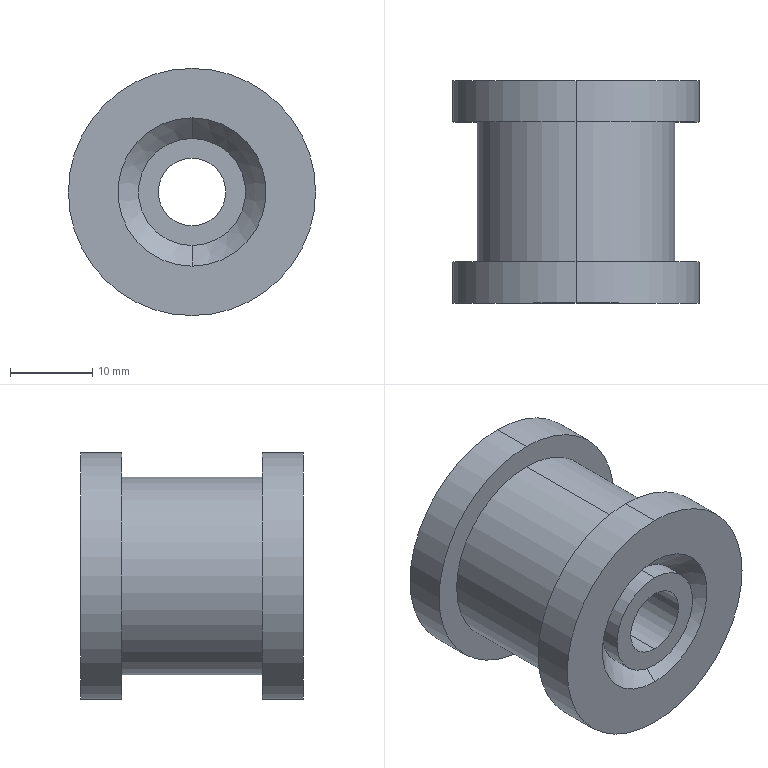Part | STEP file | B drag chain wheel | 1 solid | 22 faces | box 30 x 27 x 30 mm | volume 13045 mm3 | cylinder 12 | plane 6 | cone 4 | commonest cylinder face diameters 13 x4 30 x4 8.2 x2 24 x2
STEP:
#1=CARTESIAN_POINT('',(0.,0.,0.));
#2=DIRECTION('',(0.,0.,1.));
#3=DIRECTION('',(1.,0.,0.));
#4=AXIS2_PLACEMENT_3D('',#1,#2,#3);
#5=CARTESIAN_POINT('',(0.,27.,-4.1));
#6=VERTEX_POINT('',#5);
#7=CARTESIAN_POINT('',(0.,0.,-4.1));
#8=VERTEX_POINT('',#7);
#9=CARTESIAN_POINT('',(0.,41.,-4.1));
#10=DIRECTION('',(0.,-1.,0.));
#11=VECTOR('',#10,1.);
#12=LINE('',#9,#11);
#13=CARTESIAN_POINT('',(0.,41.,0.));
#14=DIRECTION('',(0.,-1.,0.));
#15=DIRECTION('',(0.,0.,-1.));
#16=AXIS2_PLACEMENT_3D('',#13,#14,#15);
#17=CYLINDRICAL_SURFACE('',#16,4.1);
#18=CARTESIAN_POINT('',(6.283,0.));
#19=DIRECTION('',(0.,1.));
#20=VECTOR('',#19,1.);
#21=LINE('',#18,#20);
#22=(GEOMETRIC_REPRESENTATION_CONTEXT(2)PARAMETRIC_REPRESENTATION_CONTEXT()REPRESENTATION_CONTEXT('',''));
#23=DEFINITIONAL_REPRESENTATION('',(#21),#22);
#24=PCURVE('',#17,#23);
#25=CARTESIAN_POINT('',(0.,41.,0.));
#26=DIRECTION('',(0.,-1.,0.));
#27=DIRECTION('',(0.,0.,-1.));
#28=AXIS2_PLACEMENT_3D('',#25,#26,#27);
#29=CYLINDRICAL_SURFACE('',#28,4.1);
#30=CARTESIAN_POINT('',(0.,0.));
#31=DIRECTION('',(0.,1.));
#32=VECTOR('',#31,1.);
#33=LINE('',#30,#32);
#34=(GEOMETRIC_REPRESENTATION_CONTEXT(2)PARAMETRIC_REPRESENTATION_CONTEXT()REPRESENTATION_CONTEXT('',''));
#35=DEFINITIONAL_REPRESENTATION('',(#33),#34);
#36=PCURVE('',#29,#35);
#37=SURFACE_CURVE('',#12,(#24,#36),.PCURVE_S1.);
#38=EDGE_CURVE('',#6,#8,#37,.T.);
#39=ORIENTED_EDGE('',*,*,#38,.T.);
#40=CARTESIAN_POINT('',(0.,0.,4.1));
#41=VERTEX_POINT('',#40);
#42=CARTESIAN_POINT('',(0.,0.,0.));
#43=DIRECTION('',(0.,-1.,0.));
#44=DIRECTION('',(0.,0.,-1.));
#45=AXIS2_PLACEMENT_3D('',#42,#43,#44);
#46=CIRCLE('',#45,4.1);
#47=CARTESIAN_POINT('',(0.,41.));
#48=DIRECTION('',(1.,0.));
#49=VECTOR('',#48,1.);
#50=LINE('',#47,#49);
#51=(GEOMETRIC_REPRESENTATION_CONTEXT(2)PARAMETRIC_REPRESENTATION_CONTEXT()REPRESENTATION_CONTEXT('',''));
#52=DEFINITIONAL_REPRESENTATION('',(#50),#51);
#53=PCURVE('',#17,#52);
#54=CARTESIAN_POINT('',(0.,0.,0.));
#55=DIRECTION('',(0.,-1.,0.));
#56=DIRECTION('',(0.,0.,-1.));
#57=AXIS2_PLACEMENT_3D('',#54,#55,#56);
#58=PLANE('',#57);
#59=CARTESIAN_POINT('',(0.,0.));
#60=DIRECTION('',(1.,0.));
#61=AXIS2_PLACEMENT_2D('',#59,#60);
#62=CIRCLE('',#61,4.1);
#63=(GEOMETRIC_REPRESENTATION_CONTEXT(2)PARAMETRIC_REPRESENTATION_CONTEXT()REPRESENTATION_CONTEXT('',''));
#64=DEFINITIONAL_REPRESENTATION('',(#62),#63);
#65=PCURVE('',#58,#64);
#66=SURFACE_CURVE('',#46,(#53,#65),.PCURVE_S1.);
#67=EDGE_CURVE('',#41,#8,#66,.T.);
#68=ORIENTED_EDGE('',*,*,#67,.F.);
#69=CARTESIAN_POINT('',(0.,27.,4.1));
#70=VERTEX_POINT('',#69);
#71=CARTESIAN_POINT('',(0.,41.,4.1));
#72=DIRECTION('',(0.,-1.,0.));
#73=VECTOR('',#72,1.);
#74=LINE('',#71,#73);
#75=CARTESIAN_POINT('',(3.142,0.));
#76=DIRECTION('',(0.,1.));
#77=VECTOR('',#76,1.);
#78=LINE('',#75,#77);
#79=(GEOMETRIC_REPRESENTATION_CONTEXT(2)PARAMETRIC_REPRESENTATION_CONTEXT()REPRESENTATION_CONTEXT('',''));
#80=DEFINITIONAL_REPRESENTATION('',(#78),#79);
#81=PCURVE('',#17,#80);
#82=CARTESIAN_POINT('',(3.142,0.));
#83=DIRECTION('',(0.,1.));
#84=VECTOR('',#83,1.);
#85=LINE('',#82,#84);
#86=(GEOMETRIC_REPRESENTATION_CONTEXT(2)PARAMETRIC_REPRESENTATION_CONTEXT()REPRESENTATION_CONTEXT('',''));
#87=DEFINITIONAL_REPRESENTATION('',(#85),#86);
#88=PCURVE('',#29,#87);
#89=SURFACE_CURVE('',#74,(#81,#88),.PCURVE_S1.);
#90=EDGE_CURVE('',#70,#41,#89,.T.);
#91=ORIENTED_EDGE('',*,*,#90,.F.);
#92=CARTESIAN_POINT('',(0.,27.,0.));
#93=DIRECTION('',(0.,1.,0.));
#94=DIRECTION('',(0.,0.,1.));
#95=AXIS2_PLACEMENT_3D('',#92,#93,#94);
#96=CIRCLE('',#95,4.1);
#97=CARTESIAN_POINT('',(9.425,14.));
#98=DIRECTION('',(-1.,0.));
#99=VECTOR('',#98,1.);
#100=LINE('',#97,#99);
#101=(GEOMETRIC_REPRESENTATION_CONTEXT(2)PARAMETRIC_REPRESENTATION_CONTEXT()REPRESENTATION_CONTEXT('',''));
#102=DEFINITIONAL_REPRESENTATION('',(#100),#101);
#103=PCURVE('',#17,#102);
#104=CARTESIAN_POINT('',(0.,27.,0.));
#105=DIRECTION('',(0.,1.,0.));
#106=DIRECTION('',(0.,0.,1.));
#107=AXIS2_PLACEMENT_3D('',#104,#105,#106);
#108=PLANE('',#107);
#109=CARTESIAN_POINT('',(0.,0.));
#110=DIRECTION('',(1.,0.));
#111=AXIS2_PLACEMENT_2D('',#109,#110);
#112=CIRCLE('',#111,4.1);
#113=(GEOMETRIC_REPRESENTATION_CONTEXT(2)PARAMETRIC_REPRESENTATION_CONTEXT()REPRESENTATION_CONTEXT('',''));
#114=DEFINITIONAL_REPRESENTATION('',(#112),#113);
#115=PCURVE('',#108,#114);
#116=SURFACE_CURVE('',#96,(#103,#115),.PCURVE_S1.);
#117=EDGE_CURVE('',#6,#70,#116,.T.);
#118=ORIENTED_EDGE('',*,*,#117,.F.);
#119=EDGE_LOOP('',(#39,#68,#91,#118));
#120=FACE_BOUND('',#119,.F.);
#121=ADVANCED_FACE('',(#120),#17,.F.);
#122=CARTESIAN_POINT('',(0.,27.,-6.5));
#123=VERTEX_POINT('',#122);
#124=CARTESIAN_POINT('',(0.,27.,6.5));
#125=VERTEX_POINT('',#124);
#126=CARTESIAN_POINT('',(0.,27.,0.));
#127=DIRECTION('',(0.,-1.,0.));
#128=DIRECTION('',(0.,0.,1.));
#129=AXIS2_PLACEMENT_3D('',#126,#127,#128);
#130=CIRCLE('',#129,6.5);
#131=CARTESIAN_POINT('',(0.,45.385,0.));
#132=DIRECTION('',(0.,-1.,0.));
#133=DIRECTION('',(0.,0.,-1.));
#134=AXIS2_PLACEMENT_3D('',#131,#132,#133);
#135=CYLINDRICAL_SURFACE('',#134,6.5);
#136=CARTESIAN_POINT('',(-3.142,18.385));
#137=DIRECTION('',(1.,0.));
#138=VECTOR('',#137,1.);
#139=LINE('',#136,#138);
#140=(GEOMETRIC_REPRESENTATION_CONTEXT(2)PARAMETRIC_REPRESENTATION_CONTEXT()REPRESENTATION_CONTEXT('',''));
#141=DEFINITIONAL_REPRESENTATION('',(#139),#140);
#142=PCURVE('',#135,#141);
#143=CARTESIAN_POINT('',(6.5,0.));
#144=CARTESIAN_POINT('',(6.5,-11.258));
#145=CARTESIAN_POINT('',(-3.25,-5.629));
#146=CARTESIAN_POINT('',(-13.,0.));
#147=CARTESIAN_POINT('',(-3.25,5.629));
#148=CARTESIAN_POINT('',(6.5,11.258));
#149=CARTESIAN_POINT('',(6.5,0.));
#150=(BOUNDED_CURVE()B_SPLINE_CURVE(2,(#143,#144,#145,#146,#147,#148,#149),.UNSPECIFIED.,.T.,.F.)B_SPLINE_CURVE_WITH_KNOTS((1,2,2,2,2,1),(-2.094,0.,2.094,4.189,6.283,8.378),.UNSPECIFIED.)CURVE()GEOMETRIC_REPRESENTATION_ITEM()RATIONAL_B_SPLINE_CURVE((1.,0.5,1.,0.5,1.,0.5,1.))REPRESENTATION_ITEM(''));
#151=(GEOMETRIC_REPRESENTATION_CONTEXT(2)PARAMETRIC_REPRESENTATION_CONTEXT()REPRESENTATION_CONTEXT('',''));
#152=DEFINITIONAL_REPRESENTATION('',(#150),#151);
#153=PCURVE('',#108,#152);
#154=SURFACE_CURVE('',#130,(#142,#153),.PCURVE_S1.);
#155=EDGE_CURVE('',#123,#125,#154,.T.);
#156=ORIENTED_EDGE('',*,*,#155,.T.);
#157=CARTESIAN_POINT('',(0.,24.5,6.5));
#158=VERTEX_POINT('',#157);
#159=CARTESIAN_POINT('',(0.,45.385,6.5));
#160=DIRECTION('',(0.,-1.,0.));
#161=VECTOR('',#160,1.);
#162=LINE('',#159,#161);
#163=CARTESIAN_POINT('',(3.142,0.));
#164=DIRECTION('',(0.,1.));
#165=VECTOR('',#164,1.);
#166=LINE('',#163,#165);
#167=(GEOMETRIC_REPRESENTATION_CONTEXT(2)PARAMETRIC_REPRESENTATION_CONTEXT()REPRESENTATION_CONTEXT('',''));
#168=DEFINITIONAL_REPRESENTATION('',(#166),#167);
#169=PCURVE('',#135,#168);
#170=CARTESIAN_POINT('',(0.,45.385,0.));
#171=DIRECTION('',(0.,-1.,0.));
#172=DIRECTION('',(0.,0.,-1.));
#173=AXIS2_PLACEMENT_3D('',#170,#171,#172);
#174=CYLINDRICAL_SURFACE('',#173,6.5);
#175=CARTESIAN_POINT('',(3.142,0.));
#176=DIRECTION('',(0.,1.));
#177=VECTOR('',#176,1.);
#178=LINE('',#175,#177);
#179=(GEOMETRIC_REPRESENTATION_CONTEXT(2)PARAMETRIC_REPRESENTATION_CONTEXT()REPRESENTATION_CONTEXT('',''));
#180=DEFINITIONAL_REPRESENTATION('',(#178),#179);
#181=PCURVE('',#174,#180);
#182=SURFACE_CURVE('',#162,(#169,#181),.PCURVE_S1.);
#183=EDGE_CURVE('',#125,#158,#182,.T.);
#184=ORIENTED_EDGE('',*,*,#183,.T.);
#185=CARTESIAN_POINT('',(0.,24.5,-6.5));
#186=VERTEX_POINT('',#185);
#187=CARTESIAN_POINT('',(0.,24.5,0.));
#188=DIRECTION('',(0.,1.,0.));
#189=DIRECTION('',(0.,0.,1.));
#190=AXIS2_PLACEMENT_3D('',#187,#188,#189);
#191=CIRCLE('',#190,6.5);
#192=CARTESIAN_POINT('',(3.142,20.885));
#193=DIRECTION('',(-1.,0.));
#194=VECTOR('',#193,1.);
#195=LINE('',#192,#194);
#196=(GEOMETRIC_REPRESENTATION_CONTEXT(2)PARAMETRIC_REPRESENTATION_CONTEXT()REPRESENTATION_CONTEXT('',''));
#197=DEFINITIONAL_REPRESENTATION('',(#195),#196);
#198=PCURVE('',#135,#197);
#199=CARTESIAN_POINT('',(0.,22.,0.));
#200=DIRECTION('',(0.,1.,0.));
#201=DIRECTION('',(0.,0.,1.));
#202=AXIS2_PLACEMENT_3D('',#199,#200,#201);
#203=CONICAL_SURFACE('',#202,4.,0.7854);
#204=CARTESIAN_POINT('',(0.,2.5));
#205=DIRECTION('',(1.,0.));
#206=VECTOR('',#205,1.);
#207=LINE('',#204,#206);
#208=(GEOMETRIC_REPRESENTATION_CONTEXT(2)PARAMETRIC_REPRESENTATION_CONTEXT()REPRESENTATION_CONTEXT('',''));
#209=DEFINITIONAL_REPRESENTATION('',(#207),#208);
#210=PCURVE('',#203,#209);
#211=SURFACE_CURVE('',#191,(#198,#210),.PCURVE_S1.);
#212=EDGE_CURVE('',#158,#186,#211,.T.);
#213=ORIENTED_EDGE('',*,*,#212,.T.);
#214=CARTESIAN_POINT('',(0.,45.385,-6.5));
#215=DIRECTION('',(0.,-1.,0.));
#216=VECTOR('',#215,1.);
#217=LINE('',#214,#216);
#218=CARTESIAN_POINT('',(0.,0.));
#219=DIRECTION('',(0.,1.));
#220=VECTOR('',#219,1.);
#221=LINE('',#218,#220);
#222=(GEOMETRIC_REPRESENTATION_CONTEXT(2)PARAMETRIC_REPRESENTATION_CONTEXT()REPRESENTATION_CONTEXT('',''));
#223=DEFINITIONAL_REPRESENTATION('',(#221),#222);
#224=PCURVE('',#135,#223);
#225=CARTESIAN_POINT('',(6.283,0.));
#226=DIRECTION('',(0.,1.));
#227=VECTOR('',#226,1.);
#228=LINE('',#225,#227);
#229=(GEOMETRIC_REPRESENTATION_CONTEXT(2)PARAMETRIC_REPRESENTATION_CONTEXT()REPRESENTATION_CONTEXT('',''));
#230=DEFINITIONAL_REPRESENTATION('',(#228),#229);
#231=PCURVE('',#174,#230);
#232=SURFACE_CURVE('',#217,(#224,#231),.PCURVE_S1.);
#233=EDGE_CURVE('',#123,#186,#232,.T.);
#234=ORIENTED_EDGE('',*,*,#233,.F.);
#235=EDGE_LOOP('',(#156,#184,#213,#234));
#236=FACE_BOUND('',#235,.T.);
#237=ADVANCED_FACE('',(#236),#135,.T.);
#238=CARTESIAN_POINT('',(0.,2.5,-6.5));
#239=VERTEX_POINT('',#238);
#240=CARTESIAN_POINT('',(0.,2.5,6.5));
#241=VERTEX_POINT('',#240);
#242=CARTESIAN_POINT('',(0.,2.5,0.));
#243=DIRECTION('',(0.,-1.,0.));
#244=DIRECTION('',(0.,0.,-1.));
#245=AXIS2_PLACEMENT_3D('',#242,#243,#244);
#246=CIRCLE('',#245,6.5);
#247=CARTESIAN_POINT('',(0.,45.385,0.));
#248=DIRECTION('',(0.,-1.,0.));
#249=DIRECTION('',(0.,0.,-1.));
#250=AXIS2_PLACEMENT_3D('',#247,#248,#249);
#251=CYLINDRICAL_SURFACE('',#250,6.5);
#252=CARTESIAN_POINT('',(0.,42.885));
#253=DIRECTION('',(1.,0.));
#254=VECTOR('',#253,1.);
#255=LINE('',#252,#254);
#256=(GEOMETRIC_REPRESENTATION_CONTEXT(2)PARAMETRIC_REPRESENTATION_CONTEXT()REPRESENTATION_CONTEXT('',''));
#257=DEFINITIONAL_REPRESENTATION('',(#255),#256);
#258=PCURVE('',#251,#257);
#259=CARTESIAN_POINT('',(0.,5.,0.));
#260=DIRECTION('',(0.,-1.,0.));
#261=DIRECTION('',(0.,0.,-1.));
#262=AXIS2_PLACEMENT_3D('',#259,#260,#261);
#263=CONICAL_SURFACE('',#262,4.,0.7854);
#264=CARTESIAN_POINT('',(0.,2.5));
#265=DIRECTION('',(1.,0.));
#266=VECTOR('',#265,1.);
#267=LINE('',#264,#266);
#268=(GEOMETRIC_REPRESENTATION_CONTEXT(2)PARAMETRIC_REPRESENTATION_CONTEXT()REPRESENTATION_CONTEXT('',''));
#269=DEFINITIONAL_REPRESENTATION('',(#267),#268);
#270=PCURVE('',#263,#269);
#271=SURFACE_CURVE('',#246,(#258,#270),.PCURVE_S1.);
#272=EDGE_CURVE('',#239,#241,#271,.T.);
#273=ORIENTED_EDGE('',*,*,#272,.T.);
#274=CARTESIAN_POINT('',(0.,0.,6.5));
#275=VERTEX_POINT('',#274);
#276=CARTESIAN_POINT('',(0.,45.385,6.5));
#277=DIRECTION('',(0.,-1.,0.));
#278=VECTOR('',#277,1.);
#279=LINE('',#276,#278);
#280=CARTESIAN_POINT('',(3.142,0.));
#281=DIRECTION('',(0.,1.));
#282=VECTOR('',#281,1.);
#283=LINE('',#280,#282);
#284=(GEOMETRIC_REPRESENTATION_CONTEXT(2)PARAMETRIC_REPRESENTATION_CONTEXT()REPRESENTATION_CONTEXT('',''));
#285=DEFINITIONAL_REPRESENTATION('',(#283),#284);
#286=PCURVE('',#251,#285);
#287=CARTESIAN_POINT('',(0.,45.385,0.));
#288=DIRECTION('',(0.,-1.,0.));
#289=DIRECTION('',(0.,0.,-1.));
#290=AXIS2_PLACEMENT_3D('',#287,#288,#289);
#291=CYLINDRICAL_SURFACE('',#290,6.5);
#292=CARTESIAN_POINT('',(3.142,0.));
#293=DIRECTION('',(0.,1.));
#294=VECTOR('',#293,1.);
#295=LINE('',#292,#294);
#296=(GEOMETRIC_REPRESENTATION_CONTEXT(2)PARAMETRIC_REPRESENTATION_CONTEXT()REPRESENTATION_CONTEXT('',''));
#297=DEFINITIONAL_REPRESENTATION('',(#295),#296);
#298=PCURVE('',#291,#297);
#299=SURFACE_CURVE('',#279,(#286,#298),.PCURVE_S1.);
#300=EDGE_CURVE('',#241,#275,#299,.T.);
#301=ORIENTED_EDGE('',*,*,#300,.T.);
#302=CARTESIAN_POINT('',(0.,0.,-6.5));
#303=VERTEX_POINT('',#302);
#304=CARTESIAN_POINT('',(0.,0.,0.));
#305=DIRECTION('',(0.,-1.,0.));
#306=DIRECTION('',(0.,0.,-1.));
#307=AXIS2_PLACEMENT_3D('',#304,#305,#306);
#308=CIRCLE('',#307,6.5);
#309=CARTESIAN_POINT('',(0.,45.385));
#310=DIRECTION('',(1.,0.));
#311=VECTOR('',#310,1.);
#312=LINE('',#309,#311);
#313=(GEOMETRIC_REPRESENTATION_CONTEXT(2)PARAMETRIC_REPRESENTATION_CONTEXT()REPRESENTATION_CONTEXT('',''));
#314=DEFINITIONAL_REPRESENTATION('',(#312),#313);
#315=PCURVE('',#251,#314);
#316=CARTESIAN_POINT('',(0.,0.));
#317=DIRECTION('',(1.,0.));
#318=AXIS2_PLACEMENT_2D('',#316,#317);
#319=CIRCLE('',#318,6.5);
#320=(GEOMETRIC_REPRESENTATION_CONTEXT(2)PARAMETRIC_REPRESENTATION_CONTEXT()REPRESENTATION_CONTEXT('',''));
#321=DEFINITIONAL_REPRESENTATION('',(#319),#320);
#322=PCURVE('',#58,#321);
#323=SURFACE_CURVE('',#308,(#315,#322),.PCURVE_S1.);
#324=EDGE_CURVE('',#303,#275,#323,.T.);
#325=ORIENTED_EDGE('',*,*,#324,.F.);
#326=CARTESIAN_POINT('',(0.,45.385,-6.5));
#327=DIRECTION('',(0.,-1.,0.));
#328=VECTOR('',#327,1.);
#329=LINE('',#326,#328);
#330=CARTESIAN_POINT('',(0.,0.));
#331=DIRECTION('',(0.,1.));
#332=VECTOR('',#331,1.);
#333=LINE('',#330,#332);
#334=(GEOMETRIC_REPRESENTATION_CONTEXT(2)PARAMETRIC_REPRESENTATION_CONTEXT()REPRESENTATION_CONTEXT('',''));
#335=DEFINITIONAL_REPRESENTATION('',(#333),#334);
#336=PCURVE('',#251,#335);
#337=CARTESIAN_POINT('',(6.283,0.));
#338=DIRECTION('',(0.,1.));
#339=VECTOR('',#338,1.);
#340=LINE('',#337,#339);
#341=(GEOMETRIC_REPRESENTATION_CONTEXT(2)PARAMETRIC_REPRESENTATION_CONTEXT()REPRESENTATION_CONTEXT('',''));
#342=DEFINITIONAL_REPRESENTATION('',(#340),#341);
#343=PCURVE('',#291,#342);
#344=SURFACE_CURVE('',#329,(#336,#343),.PCURVE_S1.);
#345=EDGE_CURVE('',#239,#303,#344,.T.);
#346=ORIENTED_EDGE('',*,*,#345,.F.);
#347=EDGE_LOOP('',(#273,#301,#325,#346));
#348=FACE_BOUND('',#347,.T.);
#349=ADVANCED_FACE('',(#348),#251,.T.);
#350=CARTESIAN_POINT('',(0.,27.,9.));
#351=VERTEX_POINT('',#350);
#352=CARTESIAN_POINT('',(0.,22.,4.));
#353=DIRECTION('',(0.,0.7071,0.7071));
#354=VECTOR('',#353,1.);
#355=LINE('',#352,#354);
#356=CARTESIAN_POINT('',(0.,22.,0.));
#357=DIRECTION('',(0.,1.,0.));
#358=DIRECTION('',(0.,0.,1.));
#359=AXIS2_PLACEMENT_3D('',#356,#357,#358);
#360=CONICAL_SURFACE('',#359,4.,0.7854);
#361=CARTESIAN_POINT('',(6.283,0.));
#362=DIRECTION('',(0.,1.));
#363=VECTOR('',#362,1.);
#364=LINE('',#361,#363);
#365=(GEOMETRIC_REPRESENTATION_CONTEXT(2)PARAMETRIC_REPRESENTATION_CONTEXT()REPRESENTATION_CONTEXT('',''));
#366=DEFINITIONAL_REPRESENTATION('',(#364),#365);
#367=PCURVE('',#360,#366);
#368=CARTESIAN_POINT('',(0.,0.));
#369=DIRECTION('',(0.,1.));
#370=VECTOR('',#369,1.);
#371=LINE('',#368,#370);
#372=(GEOMETRIC_REPRESENTATION_CONTEXT(2)PARAMETRIC_REPRESENTATION_CONTEXT()REPRESENTATION_CONTEXT('',''));
#373=DEFINITIONAL_REPRESENTATION('',(#371),#372);
#374=PCURVE('',#203,#373);
#375=SURFACE_CURVE('',#355,(#367,#374),.PCURVE_S1.);
#376=EDGE_CURVE('',#158,#351,#375,.T.);
#377=ORIENTED_EDGE('',*,*,#376,.T.);
#378=CARTESIAN_POINT('',(0.,27.,-9.));
#379=VERTEX_POINT('',#378);
#380=CARTESIAN_POINT('',(0.,27.,0.));
#381=DIRECTION('',(0.,-1.,0.));
#382=DIRECTION('',(0.,0.,1.));
#383=AXIS2_PLACEMENT_3D('',#380,#381,#382);
#384=CIRCLE('',#383,9.);
#385=CARTESIAN_POINT('',(6.283,5.));
#386=DIRECTION('',(-1.,0.));
#387=VECTOR('',#386,1.);
#388=LINE('',#385,#387);
#389=(GEOMETRIC_REPRESENTATION_CONTEXT(2)PARAMETRIC_REPRESENTATION_CONTEXT()REPRESENTATION_CONTEXT('',''));
#390=DEFINITIONAL_REPRESENTATION('',(#388),#389);
#391=PCURVE('',#360,#390);
#392=CARTESIAN_POINT('',(0.,27.,0.));
#393=DIRECTION('',(0.,1.,0.));
#394=DIRECTION('',(0.,0.,1.));
#395=AXIS2_PLACEMENT_3D('',#392,#393,#394);
#396=PLANE('',#395);
#397=CARTESIAN_POINT('',(9.,0.));
#398=CARTESIAN_POINT('',(9.,-15.588));
#399=CARTESIAN_POINT('',(-4.5,-7.794));
#400=CARTESIAN_POINT('',(-18.,0.));
#401=CARTESIAN_POINT('',(-4.5,7.794));
#402=CARTESIAN_POINT('',(9.,15.588));
#403=CARTESIAN_POINT('',(9.,0.));
#404=(BOUNDED_CURVE()B_SPLINE_CURVE(2,(#397,#398,#399,#400,#401,#402,#403),.UNSPECIFIED.,.T.,.F.)B_SPLINE_CURVE_WITH_KNOTS((1,2,2,2,2,1),(-2.094,0.,2.094,4.189,6.283,8.378),.UNSPECIFIED.)CURVE()GEOMETRIC_REPRESENTATION_ITEM()RATIONAL_B_SPLINE_CURVE((1.,0.5,1.,0.5,1.,0.5,1.))REPRESENTATION_ITEM(''));
#405=(GEOMETRIC_REPRESENTATION_CONTEXT(2)PARAMETRIC_REPRESENTATION_CONTEXT()REPRESENTATION_CONTEXT('',''));
#406=DEFINITIONAL_REPRESENTATION('',(#404),#405);
#407=PCURVE('',#396,#406);
#408=SURFACE_CURVE('',#384,(#391,#407),.PCURVE_S1.);
#409=EDGE_CURVE('',#351,#379,#408,.T.);
#410=ORIENTED_EDGE('',*,*,#409,.T.);
#411=CARTESIAN_POINT('',(0.,22.,-4.));
#412=DIRECTION('',(0.,0.7071,-0.7071));
#413=VECTOR('',#412,1.);
#414=LINE('',#411,#413);
#415=CARTESIAN_POINT('',(3.142,0.));
#416=DIRECTION('',(0.,1.));
#417=VECTOR('',#416,1.);
#418=LINE('',#415,#417);
#419=(GEOMETRIC_REPRESENTATION_CONTEXT(2)PARAMETRIC_REPRESENTATION_CONTEXT()REPRESENTATION_CONTEXT('',''));
#420=DEFINITIONAL_REPRESENTATION('',(#418),#419);
#421=PCURVE('',#360,#420);
#422=CARTESIAN_POINT('',(3.142,0.));
#423=DIRECTION('',(0.,1.));
#424=VECTOR('',#423,1.);
#425=LINE('',#422,#424);
#426=(GEOMETRIC_REPRESENTATION_CONTEXT(2)PARAMETRIC_REPRESENTATION_CONTEXT()REPRESENTATION_CONTEXT('',''));
#427=DEFINITIONAL_REPRESENTATION('',(#425),#426);
#428=PCURVE('',#203,#427);
#429=SURFACE_CURVE('',#414,(#421,#428),.PCURVE_S1.);
#430=EDGE_CURVE('',#186,#379,#429,.T.);
#431=ORIENTED_EDGE('',*,*,#430,.F.);
#432=CARTESIAN_POINT('',(0.,24.5,0.));
#433=DIRECTION('',(0.,1.,0.));
#434=DIRECTION('',(0.,0.,1.));
#435=AXIS2_PLACEMENT_3D('',#432,#433,#434);
#436=CIRCLE('',#435,6.5);
#437=CARTESIAN_POINT('',(0.,2.5));
#438=DIRECTION('',(1.,0.));
#439=VECTOR('',#438,1.);
#440=LINE('',#437,#439);
#441=(GEOMETRIC_REPRESENTATION_CONTEXT(2)PARAMETRIC_REPRESENTATION_CONTEXT()REPRESENTATION_CONTEXT('',''));
#442=DEFINITIONAL_REPRESENTATION('',(#440),#441);
#443=PCURVE('',#360,#442);
#444=CARTESIAN_POINT('',(9.425,20.885));
#445=DIRECTION('',(-1.,0.));
#446=VECTOR('',#445,1.);
#447=LINE('',#444,#446);
#448=(GEOMETRIC_REPRESENTATION_CONTEXT(2)PARAMETRIC_REPRESENTATION_CONTEXT()REPRESENTATION_CONTEXT('',''));
#449=DEFINITIONAL_REPRESENTATION('',(#447),#448);
#450=PCURVE('',#174,#449);
#451=SURFACE_CURVE('',#436,(#443,#450),.PCURVE_S1.);
#452=EDGE_CURVE('',#186,#158,#451,.T.);
#453=ORIENTED_EDGE('',*,*,#452,.T.);
#454=EDGE_LOOP('',(#377,#410,#431,#453));
#455=FACE_BOUND('',#454,.F.);
#456=ADVANCED_FACE('',(#455),#360,.F.);
#457=CARTESIAN_POINT('',(0.,0.,-9.));
#458=VERTEX_POINT('',#457);
#459=CARTESIAN_POINT('',(0.,5.,-4.));
#460=DIRECTION('',(0.,-0.7071,-0.7071));
#461=VECTOR('',#460,1.);
#462=LINE('',#459,#461);
#463=CARTESIAN_POINT('',(0.,5.,0.));
#464=DIRECTION('',(0.,-1.,0.));
#465=DIRECTION('',(0.,0.,-1.));
#466=AXIS2_PLACEMENT_3D('',#463,#464,#465);
#467=CONICAL_SURFACE('',#466,4.,0.7854);
#468=CARTESIAN_POINT('',(6.283,0.));
#469=DIRECTION('',(0.,1.));
#470=VECTOR('',#469,1.);
#471=LINE('',#468,#470);
#472=(GEOMETRIC_REPRESENTATION_CONTEXT(2)PARAMETRIC_REPRESENTATION_CONTEXT()REPRESENTATION_CONTEXT('',''));
#473=DEFINITIONAL_REPRESENTATION('',(#471),#472);
#474=PCURVE('',#467,#473);
#475=CARTESIAN_POINT('',(0.,0.));
#476=DIRECTION('',(0.,1.));
#477=VECTOR('',#476,1.);
#478=LINE('',#475,#477);
#479=(GEOMETRIC_REPRESENTATION_CONTEXT(2)PARAMETRIC_REPRESENTATION_CONTEXT()REPRESENTATION_CONTEXT('',''));
#480=DEFINITIONAL_REPRESENTATION('',(#478),#479);
#481=PCURVE('',#263,#480);
#482=SURFACE_CURVE('',#462,(#474,#481),.PCURVE_S1.);
#483=EDGE_CURVE('',#239,#458,#482,.T.);
#484=ORIENTED_EDGE('',*,*,#483,.T.);
#485=CARTESIAN_POINT('',(0.,0.,9.));
#486=VERTEX_POINT('',#485);
#487=CARTESIAN_POINT('',(0.,0.,0.));
#488=DIRECTION('',(0.,1.,0.));
#489=DIRECTION('',(0.,0.,1.));
#490=AXIS2_PLACEMENT_3D('',#487,#488,#489);
#491=CIRCLE('',#490,9.);
#492=CARTESIAN_POINT('',(9.425,5.));
#493=DIRECTION('',(-1.,0.));
#494=VECTOR('',#493,1.);
#495=LINE('',#492,#494);
#496=(GEOMETRIC_REPRESENTATION_CONTEXT(2)PARAMETRIC_REPRESENTATION_CONTEXT()REPRESENTATION_CONTEXT('',''));
#497=DEFINITIONAL_REPRESENTATION('',(#495),#496);
#498=PCURVE('',#467,#497);
#499=CARTESIAN_POINT('',(0.,0.,0.));
#500=DIRECTION('',(0.,1.,0.));
#501=DIRECTION('',(0.,0.,1.));
#502=AXIS2_PLACEMENT_3D('',#499,#500,#501);
#503=PLANE('',#502);
#504=CARTESIAN_POINT('',(0.,0.));
#505=DIRECTION('',(1.,0.));
#506=AXIS2_PLACEMENT_2D('',#504,#505);
#507=CIRCLE('',#506,9.);
#508=(GEOMETRIC_REPRESENTATION_CONTEXT(2)PARAMETRIC_REPRESENTATION_CONTEXT()REPRESENTATION_CONTEXT('',''));
#509=DEFINITIONAL_REPRESENTATION('',(#507),#508);
#510=PCURVE('',#503,#509);
#511=SURFACE_CURVE('',#491,(#498,#510),.PCURVE_S1.);
#512=EDGE_CURVE('',#458,#486,#511,.T.);
#513=ORIENTED_EDGE('',*,*,#512,.T.);
#514=CARTESIAN_POINT('',(0.,5.,4.));
#515=DIRECTION('',(0.,-0.7071,0.7071));
#516=VECTOR('',#515,1.);
#517=LINE('',#514,#516);
#518=CARTESIAN_POINT('',(3.142,0.));
#519=DIRECTION('',(0.,1.));
#520=VECTOR('',#519,1.);
#521=LINE('',#518,#520);
#522=(GEOMETRIC_REPRESENTATION_CONTEXT(2)PARAMETRIC_REPRESENTATION_CONTEXT()REPRESENTATION_CONTEXT('',''));
#523=DEFINITIONAL_REPRESENTATION('',(#521),#522);
#524=PCURVE('',#467,#523);
#525=CARTESIAN_POINT('',(3.142,0.));
#526=DIRECTION('',(0.,1.));
#527=VECTOR('',#526,1.);
#528=LINE('',#525,#527);
#529=(GEOMETRIC_REPRESENTATION_CONTEXT(2)PARAMETRIC_REPRESENTATION_CONTEXT()REPRESENTATION_CONTEXT('',''));
#530=DEFINITIONAL_REPRESENTATION('',(#528),#529);
#531=PCURVE('',#263,#530);
#532=SURFACE_CURVE('',#517,(#524,#531),.PCURVE_S1.);
#533=EDGE_CURVE('',#241,#486,#532,.T.);
#534=ORIENTED_EDGE('',*,*,#533,.F.);
#535=CARTESIAN_POINT('',(0.,2.5,0.));
#536=DIRECTION('',(0.,-1.,0.));
#537=DIRECTION('',(0.,0.,-1.));
#538=AXIS2_PLACEMENT_3D('',#535,#536,#537);
#539=CIRCLE('',#538,6.5);
#540=CARTESIAN_POINT('',(0.,2.5));
#541=DIRECTION('',(1.,0.));
#542=VECTOR('',#541,1.);
#543=LINE('',#540,#542);
#544=(GEOMETRIC_REPRESENTATION_CONTEXT(2)PARAMETRIC_REPRESENTATION_CONTEXT()REPRESENTATION_CONTEXT('',''));
#545=DEFINITIONAL_REPRESENTATION('',(#543),#544);
#546=PCURVE('',#467,#545);
#547=CARTESIAN_POINT('',(0.,42.885));
#548=DIRECTION('',(1.,0.));
#549=VECTOR('',#548,1.);
#550=LINE('',#547,#549);
#551=(GEOMETRIC_REPRESENTATION_CONTEXT(2)PARAMETRIC_REPRESENTATION_CONTEXT()REPRESENTATION_CONTEXT('',''));
#552=DEFINITIONAL_REPRESENTATION('',(#550),#551);
#553=PCURVE('',#291,#552);
#554=SURFACE_CURVE('',#539,(#546,#553),.PCURVE_S1.);
#555=EDGE_CURVE('',#241,#239,#554,.T.);
#556=ORIENTED_EDGE('',*,*,#555,.T.);
#557=EDGE_LOOP('',(#484,#513,#534,#556));
#558=FACE_BOUND('',#557,.F.);
#559=ADVANCED_FACE('',(#558),#467,.F.);
#560=CARTESIAN_POINT('',(0.,22.,15.));
#561=VERTEX_POINT('',#560);
#562=CARTESIAN_POINT('',(0.,22.,-15.));
#563=VERTEX_POINT('',#562);
#564=CARTESIAN_POINT('',(0.,22.,0.));
#565=DIRECTION('',(0.,1.,0.));
#566=DIRECTION('',(0.,0.,1.));
#567=AXIS2_PLACEMENT_3D('',#564,#565,#566);
#568=CIRCLE('',#567,15.);
#569=CARTESIAN_POINT('',(0.,22.,0.));
#570=DIRECTION('',(0.,1.,0.));
#571=DIRECTION('',(0.,0.,1.));
#572=AXIS2_PLACEMENT_3D('',#569,#570,#571);
#573=CYLINDRICAL_SURFACE('',#572,15.);
#574=CARTESIAN_POINT('',(0.,0.));
#575=DIRECTION('',(1.,0.));
#576=VECTOR('',#575,1.);
#577=LINE('',#574,#576);
#578=(GEOMETRIC_REPRESENTATION_CONTEXT(2)PARAMETRIC_REPRESENTATION_CONTEXT()REPRESENTATION_CONTEXT('',''));
#579=DEFINITIONAL_REPRESENTATION('',(#577),#578);
#580=PCURVE('',#573,#579);
#581=CARTESIAN_POINT('',(0.,22.,0.));
#582=DIRECTION('',(0.,1.,0.));
#583=DIRECTION('',(0.,0.,1.));
#584=AXIS2_PLACEMENT_3D('',#581,#582,#583);
#585=PLANE('',#584);
#586=CARTESIAN_POINT('',(0.,0.));
#587=DIRECTION('',(1.,0.));
#588=AXIS2_PLACEMENT_2D('',#586,#587);
#589=CIRCLE('',#588,15.);
#590=(GEOMETRIC_REPRESENTATION_CONTEXT(2)PARAMETRIC_REPRESENTATION_CONTEXT()REPRESENTATION_CONTEXT('',''));
#591=DEFINITIONAL_REPRESENTATION('',(#589),#590);
#592=PCURVE('',#585,#591);
#593=SURFACE_CURVE('',#568,(#580,#592),.PCURVE_S1.);
#594=EDGE_CURVE('',#561,#563,#593,.T.);
#595=ORIENTED_EDGE('',*,*,#594,.T.);
#596=CARTESIAN_POINT('',(0.,27.,-15.));
#597=VERTEX_POINT('',#596);
#598=CARTESIAN_POINT('',(0.,22.,-15.));
#599=DIRECTION('',(0.,1.,0.));
#600=VECTOR('',#599,1.);
#601=LINE('',#598,#600);
#602=CARTESIAN_POINT('',(3.142,0.));
#603=DIRECTION('',(0.,1.));
#604=VECTOR('',#603,1.);
#605=LINE('',#602,#604);
#606=(GEOMETRIC_REPRESENTATION_CONTEXT(2)PARAMETRIC_REPRESENTATION_CONTEXT()REPRESENTATION_CONTEXT('',''));
#607=DEFINITIONAL_REPRESENTATION('',(#605),#606);
#608=PCURVE('',#573,#607);
#609=CARTESIAN_POINT('',(0.,22.,0.));
#610=DIRECTION('',(0.,1.,0.));
#611=DIRECTION('',(0.,0.,1.));
#612=AXIS2_PLACEMENT_3D('',#609,#610,#611);
#613=CYLINDRICAL_SURFACE('',#612,15.);
#614=CARTESIAN_POINT('',(3.142,0.));
#615=DIRECTION('',(0.,1.));
#616=VECTOR('',#615,1.);
#617=LINE('',#614,#616);
#618=(GEOMETRIC_REPRESENTATION_CONTEXT(2)PARAMETRIC_REPRESENTATION_CONTEXT()REPRESENTATION_CONTEXT('',''));
#619=DEFINITIONAL_REPRESENTATION('',(#617),#618);
#620=PCURVE('',#613,#619);
#621=SURFACE_CURVE('',#601,(#608,#620),.PCURVE_S1.);
#622=EDGE_CURVE('',#563,#597,#621,.T.);
#623=ORIENTED_EDGE('',*,*,#622,.T.);
#624=CARTESIAN_POINT('',(0.,27.,15.));
#625=VERTEX_POINT('',#624);
#626=CARTESIAN_POINT('',(0.,27.,0.));
#627=DIRECTION('',(0.,1.,0.));
#628=DIRECTION('',(0.,0.,1.));
#629=AXIS2_PLACEMENT_3D('',#626,#627,#628);
#630=CIRCLE('',#629,15.);
#631=CARTESIAN_POINT('',(0.,5.));
#632=DIRECTION('',(1.,0.));
#633=VECTOR('',#632,1.);
#634=LINE('',#631,#633);
#635=(GEOMETRIC_REPRESENTATION_CONTEXT(2)PARAMETRIC_REPRESENTATION_CONTEXT()REPRESENTATION_CONTEXT('',''));
#636=DEFINITIONAL_REPRESENTATION('',(#634),#635);
#637=PCURVE('',#573,#636);
#638=CARTESIAN_POINT('',(0.,0.));
#639=DIRECTION('',(1.,0.));
#640=AXIS2_PLACEMENT_2D('',#638,#639);
#641=CIRCLE('',#640,15.);
#642=(GEOMETRIC_REPRESENTATION_CONTEXT(2)PARAMETRIC_REPRESENTATION_CONTEXT()REPRESENTATION_CONTEXT('',''));
#643=DEFINITIONAL_REPRESENTATION('',(#641),#642);
#644=PCURVE('',#396,#643);
#645=SURFACE_CURVE('',#630,(#637,#644),.PCURVE_S1.);
#646=EDGE_CURVE('',#625,#597,#645,.T.);
#647=ORIENTED_EDGE('',*,*,#646,.F.);
#648=CARTESIAN_POINT('',(0.,22.,15.));
#649=DIRECTION('',(0.,1.,0.));
#650=VECTOR('',#649,1.);
#651=LINE('',#648,#650);
#652=CARTESIAN_POINT('',(0.,0.));
#653=DIRECTION('',(0.,1.));
#654=VECTOR('',#653,1.);
#655=LINE('',#652,#654);
#656=(GEOMETRIC_REPRESENTATION_CONTEXT(2)PARAMETRIC_REPRESENTATION_CONTEXT()REPRESENTATION_CONTEXT('',''));
#657=DEFINITIONAL_REPRESENTATION('',(#655),#656);
#658=PCURVE('',#573,#657);
#659=CARTESIAN_POINT('',(6.283,0.));
#660=DIRECTION('',(0.,1.));
#661=VECTOR('',#660,1.);
#662=LINE('',#659,#661);
#663=(GEOMETRIC_REPRESENTATION_CONTEXT(2)PARAMETRIC_REPRESENTATION_CONTEXT()REPRESENTATION_CONTEXT('',''));
#664=DEFINITIONAL_REPRESENTATION('',(#662),#663);
#665=PCURVE('',#613,#664);
#666=SURFACE_CURVE('',#651,(#658,#665),.PCURVE_S1.);
#667=EDGE_CURVE('',#561,#625,#666,.T.);
#668=ORIENTED_EDGE('',*,*,#667,.F.);
#669=EDGE_LOOP('',(#595,#623,#647,#668));
#670=FACE_BOUND('',#669,.T.);
#671=ADVANCED_FACE('',(#670),#573,.T.);
#672=CARTESIAN_POINT('',(0.,5.,-15.));
#673=VERTEX_POINT('',#672);
#674=CARTESIAN_POINT('',(0.,5.,15.));
#675=VERTEX_POINT('',#674);
#676=CARTESIAN_POINT('',(0.,5.,0.));
#677=DIRECTION('',(0.,-1.,0.));
#678=DIRECTION('',(0.,0.,-1.));
#679=AXIS2_PLACEMENT_3D('',#676,#677,#678);
#680=CIRCLE('',#679,15.);
#681=CARTESIAN_POINT('',(0.,5.,0.));
#682=DIRECTION('',(0.,-1.,0.));
#683=DIRECTION('',(0.,0.,-1.));
#684=AXIS2_PLACEMENT_3D('',#681,#682,#683);
#685=CYLINDRICAL_SURFACE('',#684,15.);
#686=CARTESIAN_POINT('',(0.,0.));
#687=DIRECTION('',(1.,0.));
#688=VECTOR('',#687,1.);
#689=LINE('',#686,#688);
#690=(GEOMETRIC_REPRESENTATION_CONTEXT(2)PARAMETRIC_REPRESENTATION_CONTEXT()REPRESENTATION_CONTEXT('',''));
#691=DEFINITIONAL_REPRESENTATION('',(#689),#690);
#692=PCURVE('',#685,#691);
#693=CARTESIAN_POINT('',(0.,5.,0.));
#694=DIRECTION('',(0.,-1.,0.));
#695=DIRECTION('',(0.,0.,-1.));
#696=AXIS2_PLACEMENT_3D('',#693,#694,#695);
#697=PLANE('',#696);
#698=CARTESIAN_POINT('',(0.,0.));
#699=DIRECTION('',(1.,0.));
#700=AXIS2_PLACEMENT_2D('',#698,#699);
#701=CIRCLE('',#700,15.);
#702=(GEOMETRIC_REPRESENTATION_CONTEXT(2)PARAMETRIC_REPRESENTATION_CONTEXT()REPRESENTATION_CONTEXT('',''));
#703=DEFINITIONAL_REPRESENTATION('',(#701),#702);
#704=PCURVE('',#697,#703);
#705=SURFACE_CURVE('',#680,(#692,#704),.PCURVE_S1.);
#706=EDGE_CURVE('',#673,#675,#705,.T.);
#707=ORIENTED_EDGE('',*,*,#706,.T.);
#708=CARTESIAN_POINT('',(0.,0.,15.));
#709=VERTEX_POINT('',#708);
#710=CARTESIAN_POINT('',(0.,5.,15.));
#711=DIRECTION('',(0.,-1.,0.));
#712=VECTOR('',#711,1.);
#713=LINE('',#710,#712);
#714=CARTESIAN_POINT('',(3.142,0.));
#715=DIRECTION('',(0.,1.));
#716=VECTOR('',#715,1.);
#717=LINE('',#714,#716);
#718=(GEOMETRIC_REPRESENTATION_CONTEXT(2)PARAMETRIC_REPRESENTATION_CONTEXT()REPRESENTATION_CONTEXT('',''));
#719=DEFINITIONAL_REPRESENTATION('',(#717),#718);
#720=PCURVE('',#685,#719);
#721=CARTESIAN_POINT('',(0.,5.,0.));
#722=DIRECTION('',(0.,-1.,0.));
#723=DIRECTION('',(0.,0.,-1.));
#724=AXIS2_PLACEMENT_3D('',#721,#722,#723);
#725=CYLINDRICAL_SURFACE('',#724,15.);
#726=CARTESIAN_POINT('',(3.142,0.));
#727=DIRECTION('',(0.,1.));
#728=VECTOR('',#727,1.);
#729=LINE('',#726,#728);
#730=(GEOMETRIC_REPRESENTATION_CONTEXT(2)PARAMETRIC_REPRESENTATION_CONTEXT()REPRESENTATION_CONTEXT('',''));
#731=DEFINITIONAL_REPRESENTATION('',(#729),#730);
#732=PCURVE('',#725,#731);
#733=SURFACE_CURVE('',#713,(#720,#732),.PCURVE_S1.);
#734=EDGE_CURVE('',#675,#709,#733,.T.);
#735=ORIENTED_EDGE('',*,*,#734,.T.);
#736=CARTESIAN_POINT('',(0.,0.,-15.));
#737=VERTEX_POINT('',#736);
#738=CARTESIAN_POINT('',(0.,0.,0.));
#739=DIRECTION('',(0.,-1.,0.));
#740=DIRECTION('',(0.,0.,-1.));
#741=AXIS2_PLACEMENT_3D('',#738,#739,#740);
#742=CIRCLE('',#741,15.);
#743=CARTESIAN_POINT('',(0.,5.));
#744=DIRECTION('',(1.,0.));
#745=VECTOR('',#744,1.);
#746=LINE('',#743,#745);
#747=(GEOMETRIC_REPRESENTATION_CONTEXT(2)PARAMETRIC_REPRESENTATION_CONTEXT()REPRESENTATION_CONTEXT('',''));
#748=DEFINITIONAL_REPRESENTATION('',(#746),#747);
#749=PCURVE('',#685,#748);
#750=CARTESIAN_POINT('',(-15.,0.));
#751=CARTESIAN_POINT('',(-15.,25.981));
#752=CARTESIAN_POINT('',(7.5,12.99));
#753=CARTESIAN_POINT('',(30.,0.));
#754=CARTESIAN_POINT('',(7.5,-12.99));
#755=CARTESIAN_POINT('',(-15.,-25.981));
#756=CARTESIAN_POINT('',(-15.,0.));
#757=(BOUNDED_CURVE()B_SPLINE_CURVE(2,(#750,#751,#752,#753,#754,#755,#756),.UNSPECIFIED.,.T.,.F.)B_SPLINE_CURVE_WITH_KNOTS((1,2,2,2,2,1),(-2.094,0.,2.094,4.189,6.283,8.378),.UNSPECIFIED.)CURVE()GEOMETRIC_REPRESENTATION_ITEM()RATIONAL_B_SPLINE_CURVE((1.,0.5,1.,0.5,1.,0.5,1.))REPRESENTATION_ITEM(''));
#758=(GEOMETRIC_REPRESENTATION_CONTEXT(2)PARAMETRIC_REPRESENTATION_CONTEXT()REPRESENTATION_CONTEXT('',''));
#759=DEFINITIONAL_REPRESENTATION('',(#757),#758);
#760=PCURVE('',#503,#759);
#761=SURFACE_CURVE('',#742,(#749,#760),.PCURVE_S1.);
#762=EDGE_CURVE('',#737,#709,#761,.T.);
#763=ORIENTED_EDGE('',*,*,#762,.F.);
#764=CARTESIAN_POINT('',(0.,5.,-15.));
#765=DIRECTION('',(0.,-1.,0.));
#766=VECTOR('',#765,1.);
#767=LINE('',#764,#766);
#768=CARTESIAN_POINT('',(0.,0.));
#769=DIRECTION('',(0.,1.));
#770=VECTOR('',#769,1.);
#771=LINE('',#768,#770);
#772=(GEOMETRIC_REPRESENTATION_CONTEXT(2)PARAMETRIC_REPRESENTATION_CONTEXT()REPRESENTATION_CONTEXT('',''));
#773=DEFINITIONAL_REPRESENTATION('',(#771),#772);
#774=PCURVE('',#685,#773);
#775=CARTESIAN_POINT('',(6.283,0.));
#776=DIRECTION('',(0.,1.));
#777=VECTOR('',#776,1.);
#778=LINE('',#775,#777);
#779=(GEOMETRIC_REPRESENTATION_CONTEXT(2)PARAMETRIC_REPRESENTATION_CONTEXT()REPRESENTATION_CONTEXT('',''));
#780=DEFINITIONAL_REPRESENTATION('',(#778),#779);
#781=PCURVE('',#725,#780);
#782=SURFACE_CURVE('',#767,(#774,#781),.PCURVE_S1.);
#783=EDGE_CURVE('',#673,#737,#782,.T.);
#784=ORIENTED_EDGE('',*,*,#783,.F.);
#785=EDGE_LOOP('',(#707,#735,#763,#784));
#786=FACE_BOUND('',#785,.T.);
#787=ADVANCED_FACE('',(#786),#685,.T.);
#788=CARTESIAN_POINT('',(0.,22.,12.));
#789=VERTEX_POINT('',#788);
#790=CARTESIAN_POINT('',(0.,22.,-12.));
#791=VERTEX_POINT('',#790);
#792=CARTESIAN_POINT('',(0.,22.,0.));
#793=DIRECTION('',(0.,1.,0.));
#794=DIRECTION('',(0.,0.,1.));
#795=AXIS2_PLACEMENT_3D('',#792,#793,#794);
#796=CIRCLE('',#795,12.);
#797=CARTESIAN_POINT('',(0.,27.,0.));
#798=DIRECTION('',(0.,-1.,0.));
#799=DIRECTION('',(0.,0.,-1.));
#800=AXIS2_PLACEMENT_3D('',#797,#798,#799);
#801=CYLINDRICAL_SURFACE('',#800,12.);
#802=CARTESIAN_POINT('',(3.142,5.));
#803=DIRECTION('',(-1.,0.));
#804=VECTOR('',#803,1.);
#805=LINE('',#802,#804);
#806=(GEOMETRIC_REPRESENTATION_CONTEXT(2)PARAMETRIC_REPRESENTATION_CONTEXT()REPRESENTATION_CONTEXT('',''));
#807=DEFINITIONAL_REPRESENTATION('',(#805),#806);
#808=PCURVE('',#801,#807);
#809=CARTESIAN_POINT('',(0.,0.));
#810=DIRECTION('',(1.,0.));
#811=AXIS2_PLACEMENT_2D('',#809,#810);
#812=CIRCLE('',#811,12.);
#813=(GEOMETRIC_REPRESENTATION_CONTEXT(2)PARAMETRIC_REPRESENTATION_CONTEXT()REPRESENTATION_CONTEXT('',''));
#814=DEFINITIONAL_REPRESENTATION('',(#812),#813);
#815=PCURVE('',#585,#814);
#816=SURFACE_CURVE('',#796,(#808,#815),.PCURVE_S1.);
#817=EDGE_CURVE('',#789,#791,#816,.T.);
#818=ORIENTED_EDGE('',*,*,#817,.F.);
#819=CARTESIAN_POINT('',(0.,5.,12.));
#820=VERTEX_POINT('',#819);
#821=CARTESIAN_POINT('',(0.,27.,12.));
#822=DIRECTION('',(0.,-1.,0.));
#823=VECTOR('',#822,1.);
#824=LINE('',#821,#823);
#825=CARTESIAN_POINT('',(3.142,0.));
#826=DIRECTION('',(0.,1.));
#827=VECTOR('',#826,1.);
#828=LINE('',#825,#827);
#829=(GEOMETRIC_REPRESENTATION_CONTEXT(2)PARAMETRIC_REPRESENTATION_CONTEXT()REPRESENTATION_CONTEXT('',''));
#830=DEFINITIONAL_REPRESENTATION('',(#828),#829);
#831=PCURVE('',#801,#830);
#832=CARTESIAN_POINT('',(0.,27.,0.));
#833=DIRECTION('',(0.,-1.,0.));
#834=DIRECTION('',(0.,0.,-1.));
#835=AXIS2_PLACEMENT_3D('',#832,#833,#834);
#836=CYLINDRICAL_SURFACE('',#835,12.);
#837=CARTESIAN_POINT('',(3.142,0.));
#838=DIRECTION('',(0.,1.));
#839=VECTOR('',#838,1.);
#840=LINE('',#837,#839);
#841=(GEOMETRIC_REPRESENTATION_CONTEXT(2)PARAMETRIC_REPRESENTATION_CONTEXT()REPRESENTATION_CONTEXT('',''));
#842=DEFINITIONAL_REPRESENTATION('',(#840),#841);
#843=PCURVE('',#836,#842);
#844=SURFACE_CURVE('',#824,(#831,#843),.PCURVE_S1.);
#845=EDGE_CURVE('',#789,#820,#844,.T.);
#846=ORIENTED_EDGE('',*,*,#845,.T.);
#847=CARTESIAN_POINT('',(0.,5.,-12.));
#848=VERTEX_POINT('',#847);
#849=CARTESIAN_POINT('',(0.,5.,0.));
#850=DIRECTION('',(0.,-1.,0.));
#851=DIRECTION('',(0.,0.,-1.));
#852=AXIS2_PLACEMENT_3D('',#849,#850,#851);
#853=CIRCLE('',#852,12.);
#854=CARTESIAN_POINT('',(0.,22.));
#855=DIRECTION('',(1.,0.));
#856=VECTOR('',#855,1.);
#857=LINE('',#854,#856);
#858=(GEOMETRIC_REPRESENTATION_CONTEXT(2)PARAMETRIC_REPRESENTATION_CONTEXT()REPRESENTATION_CONTEXT('',''));
#859=DEFINITIONAL_REPRESENTATION('',(#857),#858);
#860=PCURVE('',#801,#859);
#861=CARTESIAN_POINT('',(0.,0.));
#862=DIRECTION('',(1.,0.));
#863=AXIS2_PLACEMENT_2D('',#861,#862);
#864=CIRCLE('',#863,12.);
#865=(GEOMETRIC_REPRESENTATION_CONTEXT(2)PARAMETRIC_REPRESENTATION_CONTEXT()REPRESENTATION_CONTEXT('',''));
#866=DEFINITIONAL_REPRESENTATION('',(#864),#865);
#867=PCURVE('',#697,#866);
#868=SURFACE_CURVE('',#853,(#860,#867),.PCURVE_S1.);
#869=EDGE_CURVE('',#848,#820,#868,.T.);
#870=ORIENTED_EDGE('',*,*,#869,.F.);
#871=CARTESIAN_POINT('',(0.,27.,-12.));
#872=DIRECTION('',(0.,-1.,0.));
#873=VECTOR('',#872,1.);
#874=LINE('',#871,#873);
#875=CARTESIAN_POINT('',(0.,0.));
#876=DIRECTION('',(0.,1.));
#877=VECTOR('',#876,1.);
#878=LINE('',#875,#877);
#879=(GEOMETRIC_REPRESENTATION_CONTEXT(2)PARAMETRIC_REPRESENTATION_CONTEXT()REPRESENTATION_CONTEXT('',''));
#880=DEFINITIONAL_REPRESENTATION('',(#878),#879);
#881=PCURVE('',#801,#880);
#882=CARTESIAN_POINT('',(6.283,0.));
#883=DIRECTION('',(0.,1.));
#884=VECTOR('',#883,1.);
#885=LINE('',#882,#884);
#886=(GEOMETRIC_REPRESENTATION_CONTEXT(2)PARAMETRIC_REPRESENTATION_CONTEXT()REPRESENTATION_CONTEXT('',''));
#887=DEFINITIONAL_REPRESENTATION('',(#885),#886);
#888=PCURVE('',#836,#887);
#889=SURFACE_CURVE('',#874,(#881,#888),.PCURVE_S1.);
#890=EDGE_CURVE('',#791,#848,#889,.T.);
#891=ORIENTED_EDGE('',*,*,#890,.F.);
#892=EDGE_LOOP('',(#818,#846,#870,#891));
#893=FACE_BOUND('',#892,.T.);
#894=ADVANCED_FACE('',(#893),#801,.T.);
#895=ORIENTED_EDGE('',*,*,#845,.F.);
#896=CARTESIAN_POINT('',(0.,22.,0.));
#897=DIRECTION('',(0.,1.,0.));
#898=DIRECTION('',(0.,0.,1.));
#899=AXIS2_PLACEMENT_3D('',#896,#897,#898);
#900=CIRCLE('',#899,12.);
#901=CARTESIAN_POINT('',(9.425,5.));
#902=DIRECTION('',(-1.,0.));
#903=VECTOR('',#902,1.);
#904=LINE('',#901,#903);
#905=(GEOMETRIC_REPRESENTATION_CONTEXT(2)PARAMETRIC_REPRESENTATION_CONTEXT()REPRESENTATION_CONTEXT('',''));
#906=DEFINITIONAL_REPRESENTATION('',(#904),#905);
#907=PCURVE('',#836,#906);
#908=CARTESIAN_POINT('',(0.,0.));
#909=DIRECTION('',(1.,0.));
#910=AXIS2_PLACEMENT_2D('',#908,#909);
#911=CIRCLE('',#910,12.);
#912=(GEOMETRIC_REPRESENTATION_CONTEXT(2)PARAMETRIC_REPRESENTATION_CONTEXT()REPRESENTATION_CONTEXT('',''));
#913=DEFINITIONAL_REPRESENTATION('',(#911),#912);
#914=PCURVE('',#585,#913);
#915=SURFACE_CURVE('',#900,(#907,#914),.PCURVE_S1.);
#916=EDGE_CURVE('',#791,#789,#915,.T.);
#917=ORIENTED_EDGE('',*,*,#916,.F.);
#918=ORIENTED_EDGE('',*,*,#890,.T.);
#919=CARTESIAN_POINT('',(0.,5.,0.));
#920=DIRECTION('',(0.,-1.,0.));
#921=DIRECTION('',(0.,0.,-1.));
#922=AXIS2_PLACEMENT_3D('',#919,#920,#921);
#923=CIRCLE('',#922,12.);
#924=CARTESIAN_POINT('',(0.,22.));
#925=DIRECTION('',(1.,0.));
#926=VECTOR('',#925,1.);
#927=LINE('',#924,#926);
#928=(GEOMETRIC_REPRESENTATION_CONTEXT(2)PARAMETRIC_REPRESENTATION_CONTEXT()REPRESENTATION_CONTEXT('',''));
#929=DEFINITIONAL_REPRESENTATION('',(#927),#928);
#930=PCURVE('',#836,#929);
#931=CARTESIAN_POINT('',(0.,0.));
#932=DIRECTION('',(1.,0.));
#933=AXIS2_PLACEMENT_2D('',#931,#932);
#934=CIRCLE('',#933,12.);
#935=(GEOMETRIC_REPRESENTATION_CONTEXT(2)PARAMETRIC_REPRESENTATION_CONTEXT()REPRESENTATION_CONTEXT('',''));
#936=DEFINITIONAL_REPRESENTATION('',(#934),#935);
#937=PCURVE('',#697,#936);
#938=SURFACE_CURVE('',#923,(#930,#937),.PCURVE_S1.);
#939=EDGE_CURVE('',#820,#848,#938,.T.);
#940=ORIENTED_EDGE('',*,*,#939,.F.);
#941=EDGE_LOOP('',(#895,#917,#918,#940));
#942=FACE_BOUND('',#941,.T.);
#943=ADVANCED_FACE('',(#942),#836,.T.);
#944=ORIENTED_EDGE('',*,*,#734,.F.);
#945=CARTESIAN_POINT('',(0.,5.,0.));
#946=DIRECTION('',(0.,-1.,0.));
#947=DIRECTION('',(0.,0.,-1.));
#948=AXIS2_PLACEMENT_3D('',#945,#946,#947);
#949=CIRCLE('',#948,15.);
#950=CARTESIAN_POINT('',(0.,0.));
#951=DIRECTION('',(1.,0.));
#952=VECTOR('',#951,1.);
#953=LINE('',#950,#952);
#954=(GEOMETRIC_REPRESENTATION_CONTEXT(2)PARAMETRIC_REPRESENTATION_CONTEXT()REPRESENTATION_CONTEXT('',''));
#955=DEFINITIONAL_REPRESENTATION('',(#953),#954);
#956=PCURVE('',#725,#955);
#957=CARTESIAN_POINT('',(0.,0.));
#958=DIRECTION('',(1.,0.));
#959=AXIS2_PLACEMENT_2D('',#957,#958);
#960=CIRCLE('',#959,15.);
#961=(GEOMETRIC_REPRESENTATION_CONTEXT(2)PARAMETRIC_REPRESENTATION_CONTEXT()REPRESENTATION_CONTEXT('',''));
#962=DEFINITIONAL_REPRESENTATION('',(#960),#961);
#963=PCURVE('',#697,#962);
#964=SURFACE_CURVE('',#949,(#956,#963),.PCURVE_S1.);
#965=EDGE_CURVE('',#675,#673,#964,.T.);
#966=ORIENTED_EDGE('',*,*,#965,.T.);
#967=ORIENTED_EDGE('',*,*,#783,.T.);
#968=CARTESIAN_POINT('',(0.,0.,0.));
#969=DIRECTION('',(0.,-1.,0.));
#970=DIRECTION('',(0.,0.,-1.));
#971=AXIS2_PLACEMENT_3D('',#968,#969,#970);
#972=CIRCLE('',#971,15.);
#973=CARTESIAN_POINT('',(0.,5.));
#974=DIRECTION('',(1.,0.));
#975=VECTOR('',#974,1.);
#976=LINE('',#973,#975);
#977=(GEOMETRIC_REPRESENTATION_CONTEXT(2)PARAMETRIC_REPRESENTATION_CONTEXT()REPRESENTATION_CONTEXT('',''));
#978=DEFINITIONAL_REPRESENTATION('',(#976),#977);
#979=PCURVE('',#725,#978);
#980=CARTESIAN_POINT('',(-15.,0.));
#981=CARTESIAN_POINT('',(-15.,25.981));
#982=CARTESIAN_POINT('',(7.5,12.99));
#983=CARTESIAN_POINT('',(30.,0.));
#984=CARTESIAN_POINT('',(7.5,-12.99));
#985=CARTESIAN_POINT('',(-15.,-25.981));
#986=CARTESIAN_POINT('',(-15.,0.));
#987=(BOUNDED_CURVE()B_SPLINE_CURVE(2,(#980,#981,#982,#983,#984,#985,#986),.UNSPECIFIED.,.T.,.F.)B_SPLINE_CURVE_WITH_KNOTS((1,2,2,2,2,1),(-2.094,0.,2.094,4.189,6.283,8.378),.UNSPECIFIED.)CURVE()GEOMETRIC_REPRESENTATION_ITEM()RATIONAL_B_SPLINE_CURVE((1.,0.5,1.,0.5,1.,0.5,1.))REPRESENTATION_ITEM(''));
#988=(GEOMETRIC_REPRESENTATION_CONTEXT(2)PARAMETRIC_REPRESENTATION_CONTEXT()REPRESENTATION_CONTEXT('',''));
#989=DEFINITIONAL_REPRESENTATION('',(#987),#988);
#990=PCURVE('',#503,#989);
#991=SURFACE_CURVE('',#972,(#979,#990),.PCURVE_S1.);
#992=EDGE_CURVE('',#709,#737,#991,.T.);
#993=ORIENTED_EDGE('',*,*,#992,.F.);
#994=EDGE_LOOP('',(#944,#966,#967,#993));
#995=FACE_BOUND('',#994,.T.);
#996=ADVANCED_FACE('',(#995),#725,.T.);
#997=ORIENTED_EDGE('',*,*,#869,.T.);
#998=ORIENTED_EDGE('',*,*,#939,.T.);
#999=EDGE_LOOP('',(#997,#998));
#1000=FACE_BOUND('',#999,.T.);
#1001=ORIENTED_EDGE('',*,*,#706,.F.);
#1002=ORIENTED_EDGE('',*,*,#965,.F.);
#1003=EDGE_LOOP('',(#1001,#1002));
#1004=FACE_BOUND('',#1003,.T.);
#1005=ADVANCED_FACE('',(#1000,#1004),#697,.F.);
#1006=ORIENTED_EDGE('',*,*,#512,.T.);
#1007=CARTESIAN_POINT('',(0.,0.,0.));
#1008=DIRECTION('',(0.,1.,0.));
#1009=DIRECTION('',(0.,0.,1.));
#1010=AXIS2_PLACEMENT_3D('',#1007,#1008,#1009);
#1011=CIRCLE('',#1010,9.);
#1012=CARTESIAN_POINT('',(0.,0.));
#1013=DIRECTION('',(1.,0.));
#1014=AXIS2_PLACEMENT_2D('',#1012,#1013);
#1015=CIRCLE('',#1014,9.);
#1016=(GEOMETRIC_REPRESENTATION_CONTEXT(2)PARAMETRIC_REPRESENTATION_CONTEXT()REPRESENTATION_CONTEXT('',''));
#1017=DEFINITIONAL_REPRESENTATION('',(#1015),#1016);
#1018=PCURVE('',#503,#1017);
#1019=CARTESIAN_POINT('',(3.142,5.));
#1020=DIRECTION('',(-1.,0.));
#1021=VECTOR('',#1020,1.);
#1022=LINE('',#1019,#1021);
#1023=(GEOMETRIC_REPRESENTATION_CONTEXT(2)PARAMETRIC_REPRESENTATION_CONTEXT()REPRESENTATION_CONTEXT('',''));
#1024=DEFINITIONAL_REPRESENTATION('',(#1022),#1023);
#1025=PCURVE('',#263,#1024);
#1026=SURFACE_CURVE('',#1011,(#1018,#1025),.PCURVE_S1.);
#1027=EDGE_CURVE('',#486,#458,#1026,.T.);
#1028=ORIENTED_EDGE('',*,*,#1027,.T.);
#1029=EDGE_LOOP('',(#1006,#1028));
#1030=FACE_BOUND('',#1029,.T.);
#1031=ORIENTED_EDGE('',*,*,#762,.T.);
#1032=ORIENTED_EDGE('',*,*,#992,.T.);
#1033=EDGE_LOOP('',(#1031,#1032));
#1034=FACE_BOUND('',#1033,.T.);
#1035=ADVANCED_FACE('',(#1030,#1034),#503,.F.);
#1036=ORIENTED_EDGE('',*,*,#409,.T.);
#1037=CARTESIAN_POINT('',(0.,27.,0.));
#1038=DIRECTION('',(0.,-1.,0.));
#1039=DIRECTION('',(0.,0.,1.));
#1040=AXIS2_PLACEMENT_3D('',#1037,#1038,#1039);
#1041=CIRCLE('',#1040,9.);
#1042=CARTESIAN_POINT('',(9.,0.));
#1043=CARTESIAN_POINT('',(9.,-15.588));
#1044=CARTESIAN_POINT('',(-4.5,-7.794));
#1045=CARTESIAN_POINT('',(-18.,0.));
#1046=CARTESIAN_POINT('',(-4.5,7.794));
#1047=CARTESIAN_POINT('',(9.,15.588));
#1048=CARTESIAN_POINT('',(9.,0.));
#1049=(BOUNDED_CURVE()B_SPLINE_CURVE(2,(#1042,#1043,#1044,#1045,#1046,#1047,#1048),.UNSPECIFIED.,.T.,.F.)B_SPLINE_CURVE_WITH_KNOTS((1,2,2,2,2,1),(-2.094,0.,2.094,4.189,6.283,8.378),.UNSPECIFIED.)CURVE()GEOMETRIC_REPRESENTATION_ITEM()RATIONAL_B_SPLINE_CURVE((1.,0.5,1.,0.5,1.,0.5,1.))REPRESENTATION_ITEM(''));
#1050=(GEOMETRIC_REPRESENTATION_CONTEXT(2)PARAMETRIC_REPRESENTATION_CONTEXT()REPRESENTATION_CONTEXT('',''));
#1051=DEFINITIONAL_REPRESENTATION('',(#1049),#1050);
#1052=PCURVE('',#396,#1051);
#1053=CARTESIAN_POINT('',(6.283,5.));
#1054=DIRECTION('',(-1.,0.));
#1055=VECTOR('',#1054,1.);
#1056=LINE('',#1053,#1055);
#1057=(GEOMETRIC_REPRESENTATION_CONTEXT(2)PARAMETRIC_REPRESENTATION_CONTEXT()REPRESENTATION_CONTEXT('',''));
#1058=DEFINITIONAL_REPRESENTATION('',(#1056),#1057);
#1059=PCURVE('',#203,#1058);
#1060=SURFACE_CURVE('',#1041,(#1052,#1059),.PCURVE_S1.);
#1061=EDGE_CURVE('',#379,#351,#1060,.T.);
#1062=ORIENTED_EDGE('',*,*,#1061,.T.);
#1063=EDGE_LOOP('',(#1036,#1062));
#1064=FACE_BOUND('',#1063,.T.);
#1065=ORIENTED_EDGE('',*,*,#646,.T.);
#1066=CARTESIAN_POINT('',(0.,27.,0.));
#1067=DIRECTION('',(0.,1.,0.));
#1068=DIRECTION('',(0.,0.,1.));
#1069=AXIS2_PLACEMENT_3D('',#1066,#1067,#1068);
#1070=CIRCLE('',#1069,15.);
#1071=CARTESIAN_POINT('',(0.,0.));
#1072=DIRECTION('',(1.,0.));
#1073=AXIS2_PLACEMENT_2D('',#1071,#1072);
#1074=CIRCLE('',#1073,15.);
#1075=(GEOMETRIC_REPRESENTATION_CONTEXT(2)PARAMETRIC_REPRESENTATION_CONTEXT()REPRESENTATION_CONTEXT('',''));
#1076=DEFINITIONAL_REPRESENTATION('',(#1074),#1075);
#1077=PCURVE('',#396,#1076);
#1078=CARTESIAN_POINT('',(0.,5.));
#1079=DIRECTION('',(1.,0.));
#1080=VECTOR('',#1079,1.);
#1081=LINE('',#1078,#1080);
#1082=(GEOMETRIC_REPRESENTATION_CONTEXT(2)PARAMETRIC_REPRESENTATION_CONTEXT()REPRESENTATION_CONTEXT('',''));
#1083=DEFINITIONAL_REPRESENTATION('',(#1081),#1082);
#1084=PCURVE('',#613,#1083);
#1085=SURFACE_CURVE('',#1070,(#1077,#1084),.PCURVE_S1.);
#1086=EDGE_CURVE('',#597,#625,#1085,.T.);
#1087=ORIENTED_EDGE('',*,*,#1086,.T.);
#1088=EDGE_LOOP('',(#1065,#1087));
#1089=FACE_BOUND('',#1088,.T.);
#1090=ADVANCED_FACE('',(#1064,#1089),#396,.T.);
#1091=ORIENTED_EDGE('',*,*,#622,.F.);
#1092=CARTESIAN_POINT('',(0.,22.,0.));
#1093=DIRECTION('',(0.,1.,0.));
#1094=DIRECTION('',(0.,0.,1.));
#1095=AXIS2_PLACEMENT_3D('',#1092,#1093,#1094);
#1096=CIRCLE('',#1095,15.);
#1097=CARTESIAN_POINT('',(0.,0.));
#1098=DIRECTION('',(1.,0.));
#1099=VECTOR('',#1098,1.);
#1100=LINE('',#1097,#1099);
#1101=(GEOMETRIC_REPRESENTATION_CONTEXT(2)PARAMETRIC_REPRESENTATION_CONTEXT()REPRESENTATION_CONTEXT('',''));
#1102=DEFINITIONAL_REPRESENTATION('',(#1100),#1101);
#1103=PCURVE('',#613,#1102);
#1104=CARTESIAN_POINT('',(0.,0.));
#1105=DIRECTION('',(1.,0.));
#1106=AXIS2_PLACEMENT_2D('',#1104,#1105);
#1107=CIRCLE('',#1106,15.);
#1108=(GEOMETRIC_REPRESENTATION_CONTEXT(2)PARAMETRIC_REPRESENTATION_CONTEXT()REPRESENTATION_CONTEXT('',''));
#1109=DEFINITIONAL_REPRESENTATION('',(#1107),#1108);
#1110=PCURVE('',#585,#1109);
#1111=SURFACE_CURVE('',#1096,(#1103,#1110),.PCURVE_S1.);
#1112=EDGE_CURVE('',#563,#561,#1111,.T.);
#1113=ORIENTED_EDGE('',*,*,#1112,.T.);
#1114=ORIENTED_EDGE('',*,*,#667,.T.);
#1115=ORIENTED_EDGE('',*,*,#1086,.F.);
#1116=EDGE_LOOP('',(#1091,#1113,#1114,#1115));
#1117=FACE_BOUND('',#1116,.T.);
#1118=ADVANCED_FACE('',(#1117),#613,.T.);
#1119=ORIENTED_EDGE('',*,*,#916,.T.);
#1120=ORIENTED_EDGE('',*,*,#817,.T.);
#1121=EDGE_LOOP('',(#1119,#1120));
#1122=FACE_BOUND('',#1121,.T.);
#1123=ORIENTED_EDGE('',*,*,#594,.F.);
#1124=ORIENTED_EDGE('',*,*,#1112,.F.);
#1125=EDGE_LOOP('',(#1123,#1124));
#1126=FACE_BOUND('',#1125,.T.);
#1127=ADVANCED_FACE('',(#1122,#1126),#585,.F.);
#1128=ORIENTED_EDGE('',*,*,#1027,.T.);
#1129=ORIENTED_EDGE('',*,*,#483,.F.);
#1130=ORIENTED_EDGE('',*,*,#272,.T.);
#1131=ORIENTED_EDGE('',*,*,#533,.T.);
#1132=EDGE_LOOP('',(#1128,#1129,#1130,#1131));
#1133=FACE_BOUND('',#1132,.F.);
#1134=ADVANCED_FACE('',(#1133),#263,.F.);
#1135=ORIENTED_EDGE('',*,*,#1061,.T.);
#1136=ORIENTED_EDGE('',*,*,#376,.F.);
#1137=ORIENTED_EDGE('',*,*,#212,.T.);
#1138=ORIENTED_EDGE('',*,*,#430,.T.);
#1139=EDGE_LOOP('',(#1135,#1136,#1137,#1138));
#1140=FACE_BOUND('',#1139,.F.);
#1141=ADVANCED_FACE('',(#1140),#203,.F.);
#1142=ORIENTED_EDGE('',*,*,#300,.F.);
#1143=ORIENTED_EDGE('',*,*,#555,.T.);
#1144=ORIENTED_EDGE('',*,*,#345,.T.);
#1145=CARTESIAN_POINT('',(0.,0.,0.));
#1146=DIRECTION('',(0.,-1.,0.));
#1147=DIRECTION('',(0.,0.,-1.));
#1148=AXIS2_PLACEMENT_3D('',#1145,#1146,#1147);
#1149=CIRCLE('',#1148,6.5);
#1150=CARTESIAN_POINT('',(0.,45.385));
#1151=DIRECTION('',(1.,0.));
#1152=VECTOR('',#1151,1.);
#1153=LINE('',#1150,#1152);
#1154=(GEOMETRIC_REPRESENTATION_CONTEXT(2)PARAMETRIC_REPRESENTATION_CONTEXT()REPRESENTATION_CONTEXT('',''));
#1155=DEFINITIONAL_REPRESENTATION('',(#1153),#1154);
#1156=PCURVE('',#291,#1155);
#1157=CARTESIAN_POINT('',(0.,0.));
#1158=DIRECTION('',(1.,0.));
#1159=AXIS2_PLACEMENT_2D('',#1157,#1158);
#1160=CIRCLE('',#1159,6.5);
#1161=(GEOMETRIC_REPRESENTATION_CONTEXT(2)PARAMETRIC_REPRESENTATION_CONTEXT()REPRESENTATION_CONTEXT('',''));
#1162=DEFINITIONAL_REPRESENTATION('',(#1160),#1161);
#1163=PCURVE('',#58,#1162);
#1164=SURFACE_CURVE('',#1149,(#1156,#1163),.PCURVE_S1.);
#1165=EDGE_CURVE('',#275,#303,#1164,.T.);
#1166=ORIENTED_EDGE('',*,*,#1165,.F.);
#1167=EDGE_LOOP('',(#1142,#1143,#1144,#1166));
#1168=FACE_BOUND('',#1167,.T.);
#1169=ADVANCED_FACE('',(#1168),#291,.T.);
#1170=ORIENTED_EDGE('',*,*,#183,.F.);
#1171=CARTESIAN_POINT('',(0.,27.,0.));
#1172=DIRECTION('',(0.,-1.,0.));
#1173=DIRECTION('',(0.,0.,1.));
#1174=AXIS2_PLACEMENT_3D('',#1171,#1172,#1173);
#1175=CIRCLE('',#1174,6.5);
#1176=CARTESIAN_POINT('',(3.142,18.385));
#1177=DIRECTION('',(1.,0.));
#1178=VECTOR('',#1177,1.);
#1179=LINE('',#1176,#1178);
#1180=(GEOMETRIC_REPRESENTATION_CONTEXT(2)PARAMETRIC_REPRESENTATION_CONTEXT()REPRESENTATION_CONTEXT('',''));
#1181=DEFINITIONAL_REPRESENTATION('',(#1179),#1180);
#1182=PCURVE('',#174,#1181);
#1183=CARTESIAN_POINT('',(6.5,0.));
#1184=CARTESIAN_POINT('',(6.5,-11.258));
#1185=CARTESIAN_POINT('',(-3.25,-5.629));
#1186=CARTESIAN_POINT('',(-13.,0.));
#1187=CARTESIAN_POINT('',(-3.25,5.629));
#1188=CARTESIAN_POINT('',(6.5,11.258));
#1189=CARTESIAN_POINT('',(6.5,0.));
#1190=(BOUNDED_CURVE()B_SPLINE_CURVE(2,(#1183,#1184,#1185,#1186,#1187,#1188,#1189),.UNSPECIFIED.,.T.,.F.)B_SPLINE_CURVE_WITH_KNOTS((1,2,2,2,2,1),(-2.094,0.,2.094,4.189,6.283,8.378),.UNSPECIFIED.)CURVE()GEOMETRIC_REPRESENTATION_ITEM()RATIONAL_B_SPLINE_CURVE((1.,0.5,1.,0.5,1.,0.5,1.))REPRESENTATION_ITEM(''));
#1191=(GEOMETRIC_REPRESENTATION_CONTEXT(2)PARAMETRIC_REPRESENTATION_CONTEXT()REPRESENTATION_CONTEXT('',''));
#1192=DEFINITIONAL_REPRESENTATION('',(#1190),#1191);
#1193=PCURVE('',#108,#1192);
#1194=SURFACE_CURVE('',#1175,(#1182,#1193),.PCURVE_S1.);
#1195=EDGE_CURVE('',#125,#123,#1194,.T.);
#1196=ORIENTED_EDGE('',*,*,#1195,.T.);
#1197=ORIENTED_EDGE('',*,*,#233,.T.);
#1198=ORIENTED_EDGE('',*,*,#452,.T.);
#1199=EDGE_LOOP('',(#1170,#1196,#1197,#1198));
#1200=FACE_BOUND('',#1199,.T.);
#1201=ADVANCED_FACE('',(#1200),#174,.T.);
#1202=CARTESIAN_POINT('',(0.,0.,0.));
#1203=DIRECTION('',(0.,-1.,0.));
#1204=DIRECTION('',(0.,0.,-1.));
#1205=AXIS2_PLACEMENT_3D('',#1202,#1203,#1204);
#1206=CIRCLE('',#1205,4.1);
#1207=CARTESIAN_POINT('',(0.,0.));
#1208=DIRECTION('',(1.,0.));
#1209=AXIS2_PLACEMENT_2D('',#1207,#1208);
#1210=CIRCLE('',#1209,4.1);
#1211=(GEOMETRIC_REPRESENTATION_CONTEXT(2)PARAMETRIC_REPRESENTATION_CONTEXT()REPRESENTATION_CONTEXT('',''));
#1212=DEFINITIONAL_REPRESENTATION('',(#1210),#1211);
#1213=PCURVE('',#58,#1212);
#1214=CARTESIAN_POINT('',(0.,41.));
#1215=DIRECTION('',(1.,0.));
#1216=VECTOR('',#1215,1.);
#1217=LINE('',#1214,#1216);
#1218=(GEOMETRIC_REPRESENTATION_CONTEXT(2)PARAMETRIC_REPRESENTATION_CONTEXT()REPRESENTATION_CONTEXT('',''));
#1219=DEFINITIONAL_REPRESENTATION('',(#1217),#1218);
#1220=PCURVE('',#29,#1219);
#1221=SURFACE_CURVE('',#1206,(#1213,#1220),.PCURVE_S1.);
#1222=EDGE_CURVE('',#8,#41,#1221,.T.);
#1223=ORIENTED_EDGE('',*,*,#1222,.F.);
#1224=ORIENTED_EDGE('',*,*,#67,.F.);
#1225=EDGE_LOOP('',(#1223,#1224));
#1226=FACE_BOUND('',#1225,.T.);
#1227=ORIENTED_EDGE('',*,*,#324,.T.);
#1228=ORIENTED_EDGE('',*,*,#1165,.T.);
#1229=EDGE_LOOP('',(#1227,#1228));
#1230=FACE_BOUND('',#1229,.T.);
#1231=ADVANCED_FACE('',(#1226,#1230),#58,.T.);
#1232=ORIENTED_EDGE('',*,*,#117,.F.);
#1233=CARTESIAN_POINT('',(0.,27.,0.));
#1234=DIRECTION('',(0.,1.,0.));
#1235=DIRECTION('',(0.,0.,1.));
#1236=AXIS2_PLACEMENT_3D('',#1233,#1234,#1235);
#1237=CIRCLE('',#1236,4.1);
#1238=CARTESIAN_POINT('',(0.,0.));
#1239=DIRECTION('',(1.,0.));
#1240=AXIS2_PLACEMENT_2D('',#1238,#1239);
#1241=CIRCLE('',#1240,4.1);
#1242=(GEOMETRIC_REPRESENTATION_CONTEXT(2)PARAMETRIC_REPRESENTATION_CONTEXT()REPRESENTATION_CONTEXT('',''));
#1243=DEFINITIONAL_REPRESENTATION('',(#1241),#1242);
#1244=PCURVE('',#108,#1243);
#1245=CARTESIAN_POINT('',(3.142,14.));
#1246=DIRECTION('',(-1.,0.));
#1247=VECTOR('',#1246,1.);
#1248=LINE('',#1245,#1247);
#1249=(GEOMETRIC_REPRESENTATION_CONTEXT(2)PARAMETRIC_REPRESENTATION_CONTEXT()REPRESENTATION_CONTEXT('',''));
#1250=DEFINITIONAL_REPRESENTATION('',(#1248),#1249);
#1251=PCURVE('',#29,#1250);
#1252=SURFACE_CURVE('',#1237,(#1244,#1251),.PCURVE_S1.);
#1253=EDGE_CURVE('',#70,#6,#1252,.T.);
#1254=ORIENTED_EDGE('',*,*,#1253,.F.);
#1255=EDGE_LOOP('',(#1232,#1254));
#1256=FACE_BOUND('',#1255,.T.);
#1257=ORIENTED_EDGE('',*,*,#155,.F.);
#1258=ORIENTED_EDGE('',*,*,#1195,.F.);
#1259=EDGE_LOOP('',(#1257,#1258));
#1260=FACE_BOUND('',#1259,.T.);
#1261=ADVANCED_FACE('',(#1256,#1260),#108,.T.);
#1262=ORIENTED_EDGE('',*,*,#1222,.F.);
#1263=ORIENTED_EDGE('',*,*,#38,.F.);
#1264=ORIENTED_EDGE('',*,*,#1253,.F.);
#1265=ORIENTED_EDGE('',*,*,#90,.T.);
#1266=EDGE_LOOP('',(#1262,#1263,#1264,#1265));
#1267=FACE_BOUND('',#1266,.F.);
#1268=ADVANCED_FACE('',(#1267),#29,.F.);
#1269=CLOSED_SHELL('',(#121,#237,#349,#456,#559,#671,#787,#894,#943,#996,#1005,#1035,#1090,#1118,#1127,#1134,#1141,#1169,#1201,#1231,#1261,#1268));
#1270=MANIFOLD_SOLID_BREP('',#1269);
#1271=(LENGTH_UNIT()NAMED_UNIT(*)SI_UNIT(.MILLI.,.METRE.));
#1272=UNCERTAINTY_MEASURE_WITH_UNIT(LENGTH_MEASURE(0.0000001),#1271,'','');
#1273=(NAMED_UNIT(*)PLANE_ANGLE_UNIT()SI_UNIT($,.RADIAN.));
#1274=(NAMED_UNIT(*)SI_UNIT($,.STERADIAN.)SOLID_ANGLE_UNIT());
#1275=(GEOMETRIC_REPRESENTATION_CONTEXT(3)GLOBAL_UNCERTAINTY_ASSIGNED_CONTEXT((#1272))GLOBAL_UNIT_ASSIGNED_CONTEXT((#1271,#1273,#1274))REPRESENTATION_CONTEXT('',''));
#1276=ADVANCED_BREP_SHAPE_REPRESENTATION('',(#4,#1270),#1275);